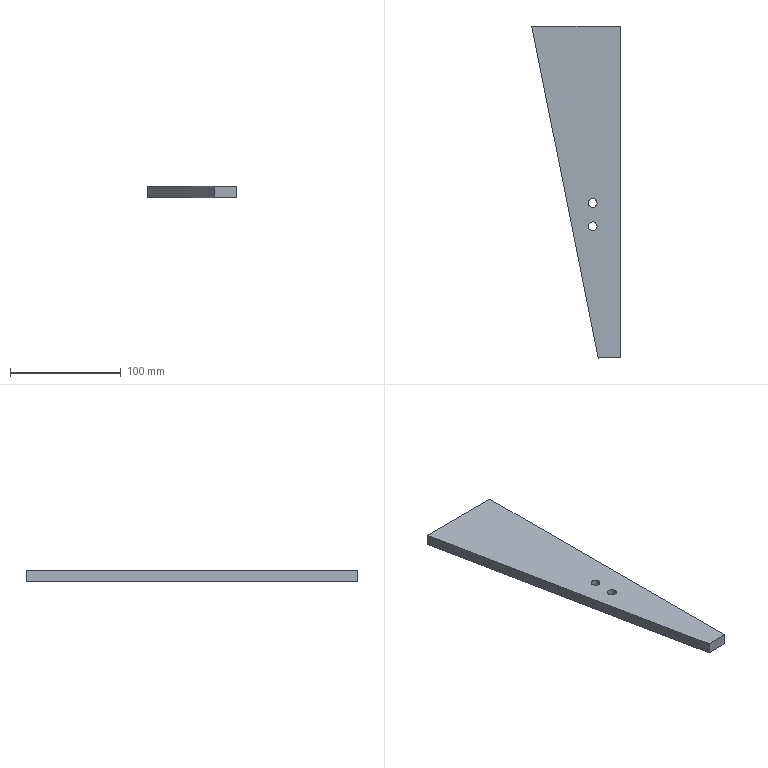Part | SolidWorks | features Extrusion 1, ICE 1 | 1 solid | 10 faces | box 80 x 300 x 10 mm | volume 148995 mm3 | plane 6 | cylinder 4 | commonest cylinder face diameters 8 x4
STEP:
#1=CARTESIAN_POINT('',(-29.,-181.,-5.));
#2=VERTEX_POINT('',#1);
#3=CARTESIAN_POINT('',(-21.,-181.,-5.));
#4=VERTEX_POINT('',#3);
#5=CARTESIAN_POINT('',(-25.,-181.,-5.));
#6=DIRECTION('',(0.,0.,1.));
#7=DIRECTION('',(1.,0.,0.));
#8=AXIS2_PLACEMENT_3D('',#5,#6,#7);
#9=CIRCLE('',#8,4.);
#10=EDGE_CURVE('',#2,#4,#9,.T.);
#11=ORIENTED_EDGE('',*,*,#10,.F.);
#12=CARTESIAN_POINT('',(-29.,-181.,5.));
#13=VERTEX_POINT('',#12);
#14=CARTESIAN_POINT('',(-29.,-181.,-5.));
#15=DIRECTION('',(0.,0.,1.));
#16=VECTOR('',#15,1000.);
#17=LINE('',#14,#16);
#18=EDGE_CURVE('',#2,#13,#17,.T.);
#19=ORIENTED_EDGE('',*,*,#18,.T.);
#20=CARTESIAN_POINT('',(-21.,-181.,5.));
#21=VERTEX_POINT('',#20);
#22=CARTESIAN_POINT('',(-25.,-181.,5.));
#23=DIRECTION('',(0.,0.,1.));
#24=DIRECTION('',(1.,0.,0.));
#25=AXIS2_PLACEMENT_3D('',#22,#23,#24);
#26=CIRCLE('',#25,4.);
#27=EDGE_CURVE('',#13,#21,#26,.T.);
#28=ORIENTED_EDGE('',*,*,#27,.T.);
#29=CARTESIAN_POINT('',(-21.,-181.,-5.));
#30=DIRECTION('',(0.,0.,1.));
#31=VECTOR('',#30,1000.);
#32=LINE('',#29,#31);
#33=EDGE_CURVE('',#4,#21,#32,.T.);
#34=ORIENTED_EDGE('',*,*,#33,.F.);
#35=EDGE_LOOP('',(#11,#19,#28,#34));
#36=FACE_OUTER_BOUND('',#35,.T.);
#37=CARTESIAN_POINT('',(-25.,-181.,-5.));
#38=DIRECTION('',(0.,0.,1.));
#39=DIRECTION('',(1.,0.,0.));
#40=AXIS2_PLACEMENT_3D('',#37,#38,#39);
#41=CYLINDRICAL_SURFACE('',#40,4.);
#42=ADVANCED_FACE('',(#36),#41,.F.);
#43=CARTESIAN_POINT('',(-29.,-160.,-5.));
#44=VERTEX_POINT('',#43);
#45=CARTESIAN_POINT('',(-21.,-160.,-5.));
#46=VERTEX_POINT('',#45);
#47=CARTESIAN_POINT('',(-25.,-160.,-5.));
#48=DIRECTION('',(0.,0.,1.));
#49=DIRECTION('',(1.,0.,0.));
#50=AXIS2_PLACEMENT_3D('',#47,#48,#49);
#51=CIRCLE('',#50,4.);
#52=EDGE_CURVE('',#44,#46,#51,.T.);
#53=ORIENTED_EDGE('',*,*,#52,.F.);
#54=CARTESIAN_POINT('',(-29.,-160.,5.));
#55=VERTEX_POINT('',#54);
#56=CARTESIAN_POINT('',(-29.,-160.,-5.));
#57=DIRECTION('',(0.,0.,1.));
#58=VECTOR('',#57,1000.);
#59=LINE('',#56,#58);
#60=EDGE_CURVE('',#44,#55,#59,.T.);
#61=ORIENTED_EDGE('',*,*,#60,.T.);
#62=CARTESIAN_POINT('',(-21.,-160.,5.));
#63=VERTEX_POINT('',#62);
#64=CARTESIAN_POINT('',(-25.,-160.,5.));
#65=DIRECTION('',(0.,0.,1.));
#66=DIRECTION('',(1.,0.,0.));
#67=AXIS2_PLACEMENT_3D('',#64,#65,#66);
#68=CIRCLE('',#67,4.);
#69=EDGE_CURVE('',#55,#63,#68,.T.);
#70=ORIENTED_EDGE('',*,*,#69,.T.);
#71=CARTESIAN_POINT('',(-21.,-160.,-5.));
#72=DIRECTION('',(0.,0.,1.));
#73=VECTOR('',#72,1000.);
#74=LINE('',#71,#73);
#75=EDGE_CURVE('',#46,#63,#74,.T.);
#76=ORIENTED_EDGE('',*,*,#75,.F.);
#77=EDGE_LOOP('',(#53,#61,#70,#76));
#78=FACE_OUTER_BOUND('',#77,.T.);
#79=CARTESIAN_POINT('',(-25.,-160.,-5.));
#80=DIRECTION('',(0.,0.,1.));
#81=DIRECTION('',(1.,0.,0.));
#82=AXIS2_PLACEMENT_3D('',#79,#80,#81);
#83=CYLINDRICAL_SURFACE('',#82,4.);
#84=ADVANCED_FACE('',(#78),#83,.F.);
#85=CARTESIAN_POINT('',(-80.,0.,-5.));
#86=VERTEX_POINT('',#85);
#87=CARTESIAN_POINT('',(-20.,-300.,-5.));
#88=VERTEX_POINT('',#87);
#89=CARTESIAN_POINT('',(-20.,-300.,-5.));
#90=DIRECTION('',(0.1961,-0.9806,0.));
#91=VECTOR('',#90,1000.);
#92=LINE('',#89,#91);
#93=EDGE_CURVE('',#86,#88,#92,.T.);
#94=ORIENTED_EDGE('',*,*,#93,.T.);
#95=CARTESIAN_POINT('',(-20.,-300.,5.));
#96=VERTEX_POINT('',#95);
#97=CARTESIAN_POINT('',(-20.,-300.,5.));
#98=DIRECTION('',(0.,0.,-1.));
#99=VECTOR('',#98,1000.);
#100=LINE('',#97,#99);
#101=EDGE_CURVE('',#96,#88,#100,.T.);
#102=ORIENTED_EDGE('',*,*,#101,.F.);
#103=CARTESIAN_POINT('',(-80.,0.,5.));
#104=VERTEX_POINT('',#103);
#105=CARTESIAN_POINT('',(-20.,-300.,5.));
#106=DIRECTION('',(0.1961,-0.9806,0.));
#107=VECTOR('',#106,1000.);
#108=LINE('',#105,#107);
#109=EDGE_CURVE('',#104,#96,#108,.T.);
#110=ORIENTED_EDGE('',*,*,#109,.F.);
#111=CARTESIAN_POINT('',(-80.,0.,5.));
#112=DIRECTION('',(0.,0.,-1.));
#113=VECTOR('',#112,1000.);
#114=LINE('',#111,#113);
#115=EDGE_CURVE('',#104,#86,#114,.T.);
#116=ORIENTED_EDGE('',*,*,#115,.T.);
#117=EDGE_LOOP('',(#94,#102,#110,#116));
#118=FACE_OUTER_BOUND('',#117,.T.);
#119=CARTESIAN_POINT('',(-20.,-300.,5.));
#120=DIRECTION('',(0.9806,0.1961,0.));
#121=DIRECTION('',(-0.1961,0.9806,0.));
#122=AXIS2_PLACEMENT_3D('',#119,#120,#121);
#123=PLANE('',#122);
#124=ADVANCED_FACE('',(#118),#123,.F.);
#125=CARTESIAN_POINT('',(0.,-300.,-5.));
#126=VERTEX_POINT('',#125);
#127=CARTESIAN_POINT('',(0.,-300.,-5.));
#128=DIRECTION('',(1.,0.,0.));
#129=VECTOR('',#128,1000.);
#130=LINE('',#127,#129);
#131=EDGE_CURVE('',#88,#126,#130,.T.);
#132=ORIENTED_EDGE('',*,*,#131,.T.);
#133=CARTESIAN_POINT('',(0.,-300.,5.));
#134=VERTEX_POINT('',#133);
#135=CARTESIAN_POINT('',(0.,-300.,5.));
#136=DIRECTION('',(0.,0.,-1.));
#137=VECTOR('',#136,1000.);
#138=LINE('',#135,#137);
#139=EDGE_CURVE('',#134,#126,#138,.T.);
#140=ORIENTED_EDGE('',*,*,#139,.F.);
#141=CARTESIAN_POINT('',(0.,-300.,5.));
#142=DIRECTION('',(1.,0.,0.));
#143=VECTOR('',#142,1000.);
#144=LINE('',#141,#143);
#145=EDGE_CURVE('',#96,#134,#144,.T.);
#146=ORIENTED_EDGE('',*,*,#145,.F.);
#147=ORIENTED_EDGE('',*,*,#101,.T.);
#148=EDGE_LOOP('',(#132,#140,#146,#147));
#149=FACE_OUTER_BOUND('',#148,.T.);
#150=CARTESIAN_POINT('',(0.,-300.,5.));
#151=DIRECTION('',(0.,1.,0.));
#152=DIRECTION('',(0.,0.,1.));
#153=AXIS2_PLACEMENT_3D('',#150,#151,#152);
#154=PLANE('',#153);
#155=ADVANCED_FACE('',(#149),#154,.F.);
#156=CARTESIAN_POINT('',(0.,0.,-5.));
#157=VERTEX_POINT('',#156);
#158=CARTESIAN_POINT('',(0.,0.,-5.));
#159=DIRECTION('',(0.,1.,0.));
#160=VECTOR('',#159,1000.);
#161=LINE('',#158,#160);
#162=EDGE_CURVE('',#126,#157,#161,.T.);
#163=ORIENTED_EDGE('',*,*,#162,.T.);
#164=CARTESIAN_POINT('',(0.,0.,5.));
#165=VERTEX_POINT('',#164);
#166=CARTESIAN_POINT('',(0.,0.,5.));
#167=DIRECTION('',(0.,0.,-1.));
#168=VECTOR('',#167,1000.);
#169=LINE('',#166,#168);
#170=EDGE_CURVE('',#165,#157,#169,.T.);
#171=ORIENTED_EDGE('',*,*,#170,.F.);
#172=CARTESIAN_POINT('',(0.,0.,5.));
#173=DIRECTION('',(0.,1.,0.));
#174=VECTOR('',#173,1000.);
#175=LINE('',#172,#174);
#176=EDGE_CURVE('',#134,#165,#175,.T.);
#177=ORIENTED_EDGE('',*,*,#176,.F.);
#178=ORIENTED_EDGE('',*,*,#139,.T.);
#179=EDGE_LOOP('',(#163,#171,#177,#178));
#180=FACE_OUTER_BOUND('',#179,.T.);
#181=CARTESIAN_POINT('',(0.,0.,5.));
#182=DIRECTION('',(-1.,0.,0.));
#183=DIRECTION('',(0.,-1.,0.));
#184=AXIS2_PLACEMENT_3D('',#181,#182,#183);
#185=PLANE('',#184);
#186=ADVANCED_FACE('',(#180),#185,.F.);
#187=CARTESIAN_POINT('',(-80.,0.,-5.));
#188=DIRECTION('',(-1.,0.,0.));
#189=VECTOR('',#188,1000.);
#190=LINE('',#187,#189);
#191=EDGE_CURVE('',#157,#86,#190,.T.);
#192=ORIENTED_EDGE('',*,*,#191,.T.);
#193=ORIENTED_EDGE('',*,*,#115,.F.);
#194=CARTESIAN_POINT('',(-80.,0.,5.));
#195=DIRECTION('',(-1.,0.,0.));
#196=VECTOR('',#195,1000.);
#197=LINE('',#194,#196);
#198=EDGE_CURVE('',#165,#104,#197,.T.);
#199=ORIENTED_EDGE('',*,*,#198,.F.);
#200=ORIENTED_EDGE('',*,*,#170,.T.);
#201=EDGE_LOOP('',(#192,#193,#199,#200));
#202=FACE_OUTER_BOUND('',#201,.T.);
#203=CARTESIAN_POINT('',(-80.,0.,5.));
#204=DIRECTION('',(0.,-1.,0.));
#205=DIRECTION('',(0.,0.,-1.));
#206=AXIS2_PLACEMENT_3D('',#203,#204,#205);
#207=PLANE('',#206);
#208=ADVANCED_FACE('',(#202),#207,.F.);
#209=CARTESIAN_POINT('',(-25.,-181.,5.));
#210=DIRECTION('',(0.,0.,1.));
#211=DIRECTION('',(1.,0.,0.));
#212=AXIS2_PLACEMENT_3D('',#209,#210,#211);
#213=CIRCLE('',#212,4.);
#214=EDGE_CURVE('',#21,#13,#213,.T.);
#215=ORIENTED_EDGE('',*,*,#214,.F.);
#216=ORIENTED_EDGE('',*,*,#27,.F.);
#217=EDGE_LOOP('',(#215,#216));
#218=FACE_BOUND('',#217,.T.);
#219=CARTESIAN_POINT('',(-25.,-160.,5.));
#220=DIRECTION('',(0.,0.,1.));
#221=DIRECTION('',(1.,0.,0.));
#222=AXIS2_PLACEMENT_3D('',#219,#220,#221);
#223=CIRCLE('',#222,4.);
#224=EDGE_CURVE('',#63,#55,#223,.T.);
#225=ORIENTED_EDGE('',*,*,#224,.F.);
#226=ORIENTED_EDGE('',*,*,#69,.F.);
#227=EDGE_LOOP('',(#225,#226));
#228=FACE_BOUND('',#227,.T.);
#229=ORIENTED_EDGE('',*,*,#109,.T.);
#230=ORIENTED_EDGE('',*,*,#145,.T.);
#231=ORIENTED_EDGE('',*,*,#176,.T.);
#232=ORIENTED_EDGE('',*,*,#198,.T.);
#233=EDGE_LOOP('',(#229,#230,#231,#232));
#234=FACE_OUTER_BOUND('',#233,.T.);
#235=CARTESIAN_POINT('',(-80.,0.,5.));
#236=DIRECTION('',(0.,0.,-1.));
#237=DIRECTION('',(-1.,0.,0.));
#238=AXIS2_PLACEMENT_3D('',#235,#236,#237);
#239=PLANE('',#238);
#240=ADVANCED_FACE('',(#218,#228,#234),#239,.F.);
#241=CARTESIAN_POINT('',(-25.,-181.,-5.));
#242=DIRECTION('',(0.,0.,1.));
#243=DIRECTION('',(1.,0.,0.));
#244=AXIS2_PLACEMENT_3D('',#241,#242,#243);
#245=CIRCLE('',#244,4.);
#246=EDGE_CURVE('',#4,#2,#245,.T.);
#247=ORIENTED_EDGE('',*,*,#246,.T.);
#248=ORIENTED_EDGE('',*,*,#10,.T.);
#249=EDGE_LOOP('',(#247,#248));
#250=FACE_BOUND('',#249,.T.);
#251=CARTESIAN_POINT('',(-25.,-160.,-5.));
#252=DIRECTION('',(0.,0.,1.));
#253=DIRECTION('',(1.,0.,0.));
#254=AXIS2_PLACEMENT_3D('',#251,#252,#253);
#255=CIRCLE('',#254,4.);
#256=EDGE_CURVE('',#46,#44,#255,.T.);
#257=ORIENTED_EDGE('',*,*,#256,.T.);
#258=ORIENTED_EDGE('',*,*,#52,.T.);
#259=EDGE_LOOP('',(#257,#258));
#260=FACE_BOUND('',#259,.T.);
#261=ORIENTED_EDGE('',*,*,#93,.F.);
#262=ORIENTED_EDGE('',*,*,#191,.F.);
#263=ORIENTED_EDGE('',*,*,#162,.F.);
#264=ORIENTED_EDGE('',*,*,#131,.F.);
#265=EDGE_LOOP('',(#261,#262,#263,#264));
#266=FACE_OUTER_BOUND('',#265,.T.);
#267=CARTESIAN_POINT('',(-80.,0.,-5.));
#268=DIRECTION('',(0.,0.,-1.));
#269=DIRECTION('',(-1.,0.,0.));
#270=AXIS2_PLACEMENT_3D('',#267,#268,#269);
#271=PLANE('',#270);
#272=ADVANCED_FACE('',(#250,#260,#266),#271,.T.);
#273=ORIENTED_EDGE('',*,*,#60,.F.);
#274=ORIENTED_EDGE('',*,*,#256,.F.);
#275=ORIENTED_EDGE('',*,*,#75,.T.);
#276=ORIENTED_EDGE('',*,*,#224,.T.);
#277=EDGE_LOOP('',(#273,#274,#275,#276));
#278=FACE_OUTER_BOUND('',#277,.T.);
#279=CARTESIAN_POINT('',(-25.,-160.,-5.));
#280=DIRECTION('',(0.,0.,1.));
#281=DIRECTION('',(1.,0.,0.));
#282=AXIS2_PLACEMENT_3D('',#279,#280,#281);
#283=CYLINDRICAL_SURFACE('',#282,4.);
#284=ADVANCED_FACE('',(#278),#283,.F.);
#285=ORIENTED_EDGE('',*,*,#18,.F.);
#286=ORIENTED_EDGE('',*,*,#246,.F.);
#287=ORIENTED_EDGE('',*,*,#33,.T.);
#288=ORIENTED_EDGE('',*,*,#214,.T.);
#289=EDGE_LOOP('',(#285,#286,#287,#288));
#290=FACE_OUTER_BOUND('',#289,.T.);
#291=CARTESIAN_POINT('',(-25.,-181.,-5.));
#292=DIRECTION('',(0.,0.,1.));
#293=DIRECTION('',(1.,0.,0.));
#294=AXIS2_PLACEMENT_3D('',#291,#292,#293);
#295=CYLINDRICAL_SURFACE('',#294,4.);
#296=ADVANCED_FACE('',(#290),#295,.F.);
#297=CLOSED_SHELL('',(#42,#84,#124,#155,#186,#208,#240,#272,#284,#296));
#298=MANIFOLD_SOLID_BREP('',#297);
#299=CARTESIAN_POINT('',(0.,0.,0.));
#300=DIRECTION('',(0.,0.,1.));
#301=DIRECTION('',(1.,0.,0.));
#302=AXIS2_PLACEMENT_3D('',#299,#300,#301);
#303=(LENGTH_UNIT()NAMED_UNIT(*)SI_UNIT(.MILLI.,.METRE.));
#304=UNCERTAINTY_MEASURE_WITH_UNIT(LENGTH_MEASURE(0.00001),#303,'','');
#305=(NAMED_UNIT(*)PLANE_ANGLE_UNIT()SI_UNIT($,.RADIAN.));
#306=(NAMED_UNIT(*)SI_UNIT($,.STERADIAN.)SOLID_ANGLE_UNIT());
#307=(GEOMETRIC_REPRESENTATION_CONTEXT(3)GLOBAL_UNCERTAINTY_ASSIGNED_CONTEXT((#304))GLOBAL_UNIT_ASSIGNED_CONTEXT((#303,#305,#306))REPRESENTATION_CONTEXT('',''));
#308=ADVANCED_BREP_SHAPE_REPRESENTATION('',(#298,#302),#307);